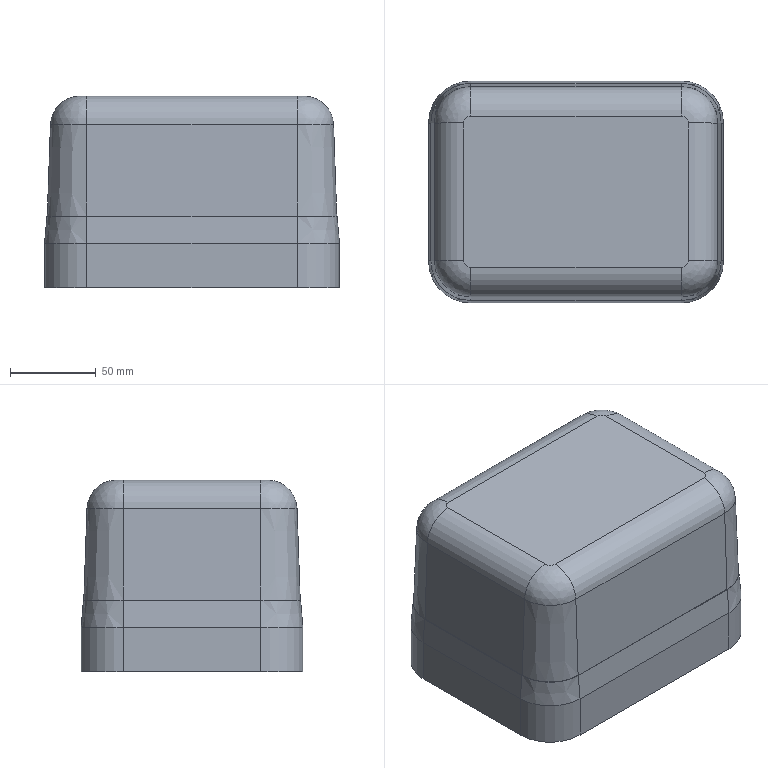Part | STEP file | SL2-MOLD_id718_xmt_txt | 1 solid | 166 faces | box 172.262 x 129.59 x 111.89 mm | volume 1963711 mm3 | plane 72 | cylinder 69 | cone 21 | spline 4 | commonest cylinder face diameters 20 x26 16 x13 10 x6 24 x6 29.4 x6 12 x4